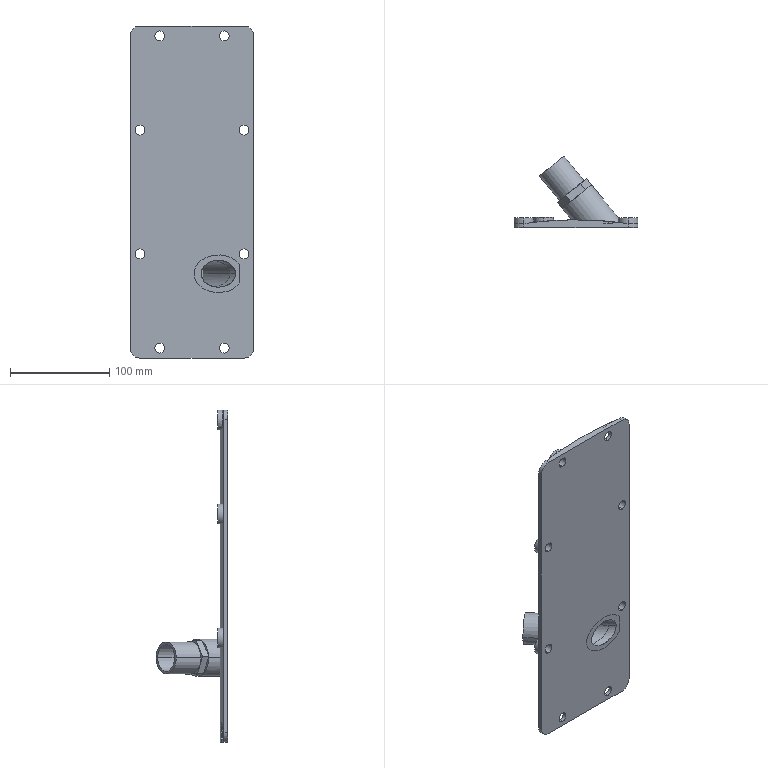Part | SolidWorks | features BaseBody 3 | 3 solids | 79 faces | box 125 x 72.421 x 335 mm | volume 284054 mm3 | cylinder 45 | plane 32 | spline 2 | commonest cylinder face diameters 10 x16 20 x14 19.9 x6 27 x4 32 x2 38 x2